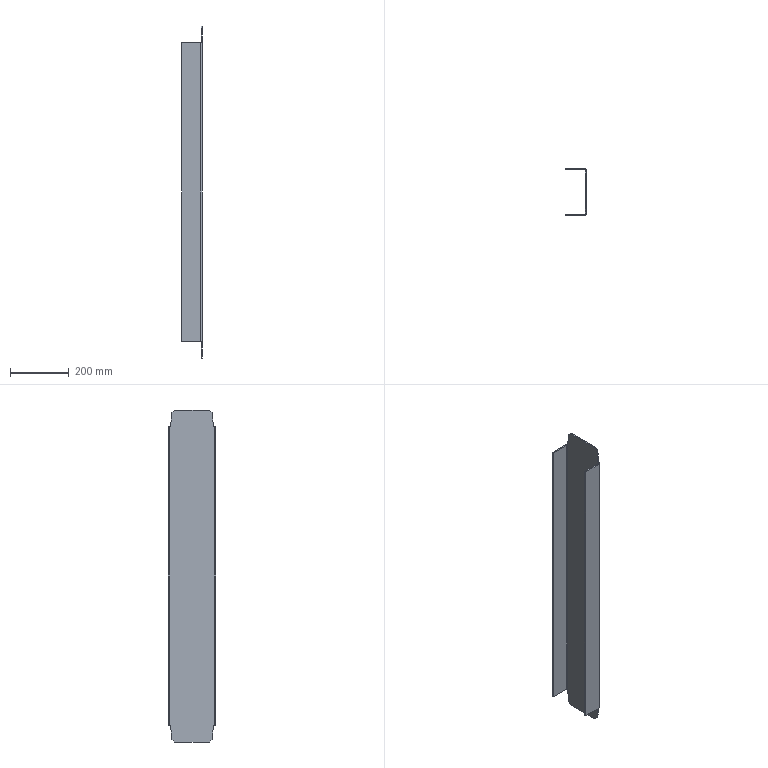Part | SolidWorks | 1 solid | 38 faces | box 70 x 160 x 1127 mm | volume 1236525 mm3 | plane 34 | cylinder 4 | commonest cylinder face diameters 2 x2 10 x2
STEP:
#1=CARTESIAN_POINT('',(-70.,4.,-507.));
#2=VERTEX_POINT('',#1);
#3=CARTESIAN_POINT('',(-5.,4.,-507.));
#4=VERTEX_POINT('',#3);
#5=CARTESIAN_POINT('',(0.,4.,-507.));
#6=DIRECTION('',(1.,0.,0.));
#7=VECTOR('',#6,1000.);
#8=LINE('',#5,#7);
#9=EDGE_CURVE('',#2,#4,#8,.T.);
#10=ORIENTED_EDGE('',*,*,#9,.F.);
#11=CARTESIAN_POINT('',(-70.,4.,507.));
#12=VERTEX_POINT('',#11);
#13=CARTESIAN_POINT('',(-70.,4.,563.5));
#14=DIRECTION('',(0.,0.,-1.));
#15=VECTOR('',#14,1000.);
#16=LINE('',#13,#15);
#17=EDGE_CURVE('',#12,#2,#16,.T.);
#18=ORIENTED_EDGE('',*,*,#17,.F.);
#19=CARTESIAN_POINT('',(-5.,4.,507.));
#20=VERTEX_POINT('',#19);
#21=CARTESIAN_POINT('',(0.,4.,507.));
#22=DIRECTION('',(1.,0.,0.));
#23=VECTOR('',#22,1000.);
#24=LINE('',#21,#23);
#25=EDGE_CURVE('',#12,#20,#24,.T.);
#26=ORIENTED_EDGE('',*,*,#25,.T.);
#27=CARTESIAN_POINT('',(-5.,4.,563.5));
#28=DIRECTION('',(0.,0.,-1.));
#29=VECTOR('',#28,1000.);
#30=LINE('',#27,#29);
#31=EDGE_CURVE('',#20,#4,#30,.T.);
#32=ORIENTED_EDGE('',*,*,#31,.T.);
#33=EDGE_LOOP('',(#10,#18,#26,#32));
#34=FACE_OUTER_BOUND('',#33,.T.);
#35=CARTESIAN_POINT('',(0.,4.,563.5));
#36=DIRECTION('',(0.,-1.,0.));
#37=DIRECTION('',(1.,0.,0.));
#38=AXIS2_PLACEMENT_3D('',#35,#36,#37);
#39=PLANE('',#38);
#40=ADVANCED_FACE('',(#34),#39,.F.);
#41=ORIENTED_EDGE('',*,*,#17,.T.);
#42=CARTESIAN_POINT('',(-70.,0.,-507.));
#43=VERTEX_POINT('',#42);
#44=CARTESIAN_POINT('',(-70.,0.,-507.));
#45=DIRECTION('',(0.,1.,0.));
#46=VECTOR('',#45,1000.);
#47=LINE('',#44,#46);
#48=EDGE_CURVE('',#43,#2,#47,.T.);
#49=ORIENTED_EDGE('',*,*,#48,.F.);
#50=CARTESIAN_POINT('',(-70.,0.,507.));
#51=VERTEX_POINT('',#50);
#52=CARTESIAN_POINT('',(-70.,0.,563.5));
#53=DIRECTION('',(0.,0.,-1.));
#54=VECTOR('',#53,1000.);
#55=LINE('',#52,#54);
#56=EDGE_CURVE('',#51,#43,#55,.T.);
#57=ORIENTED_EDGE('',*,*,#56,.F.);
#58=CARTESIAN_POINT('',(-70.,0.,507.));
#59=DIRECTION('',(0.,1.,0.));
#60=VECTOR('',#59,1000.);
#61=LINE('',#58,#60);
#62=EDGE_CURVE('',#51,#12,#61,.T.);
#63=ORIENTED_EDGE('',*,*,#62,.T.);
#64=EDGE_LOOP('',(#41,#49,#57,#63));
#65=FACE_OUTER_BOUND('',#64,.T.);
#66=CARTESIAN_POINT('',(-70.,0.,563.5));
#67=DIRECTION('',(-1.,0.,0.));
#68=DIRECTION('',(0.,0.,1.));
#69=AXIS2_PLACEMENT_3D('',#66,#67,#68);
#70=PLANE('',#69);
#71=ADVANCED_FACE('',(#65),#70,.T.);
#72=ORIENTED_EDGE('',*,*,#56,.T.);
#73=CARTESIAN_POINT('',(-5.,0.,-507.));
#74=VERTEX_POINT('',#73);
#75=CARTESIAN_POINT('',(0.,0.,-507.));
#76=DIRECTION('',(1.,0.,0.));
#77=VECTOR('',#76,1000.);
#78=LINE('',#75,#77);
#79=EDGE_CURVE('',#43,#74,#78,.T.);
#80=ORIENTED_EDGE('',*,*,#79,.T.);
#81=CARTESIAN_POINT('',(-5.,0.,507.));
#82=VERTEX_POINT('',#81);
#83=CARTESIAN_POINT('',(-5.,0.,563.5));
#84=DIRECTION('',(0.,0.,-1.));
#85=VECTOR('',#84,1000.);
#86=LINE('',#83,#85);
#87=EDGE_CURVE('',#82,#74,#86,.T.);
#88=ORIENTED_EDGE('',*,*,#87,.F.);
#89=CARTESIAN_POINT('',(0.,0.,507.));
#90=DIRECTION('',(1.,0.,0.));
#91=VECTOR('',#90,1000.);
#92=LINE('',#89,#91);
#93=EDGE_CURVE('',#51,#82,#92,.T.);
#94=ORIENTED_EDGE('',*,*,#93,.F.);
#95=EDGE_LOOP('',(#72,#80,#88,#94));
#96=FACE_OUTER_BOUND('',#95,.T.);
#97=CARTESIAN_POINT('',(0.,0.,563.5));
#98=DIRECTION('',(0.,-1.,0.));
#99=DIRECTION('',(1.,0.,0.));
#100=AXIS2_PLACEMENT_3D('',#97,#98,#99);
#101=PLANE('',#100);
#102=ADVANCED_FACE('',(#96),#101,.T.);
#103=ORIENTED_EDGE('',*,*,#87,.T.);
#104=CARTESIAN_POINT('',(0.,5.,-507.));
#105=VERTEX_POINT('',#104);
#106=CARTESIAN_POINT('',(-5.,5.,-507.));
#107=DIRECTION('',(0.,0.,1.));
#108=DIRECTION('',(0.,1.,0.));
#109=AXIS2_PLACEMENT_3D('',#106,#107,#108);
#110=CIRCLE('',#109,5.);
#111=EDGE_CURVE('',#74,#105,#110,.T.);
#112=ORIENTED_EDGE('',*,*,#111,.T.);
#113=CARTESIAN_POINT('',(0.,5.,507.));
#114=VERTEX_POINT('',#113);
#115=CARTESIAN_POINT('',(0.,5.,563.5));
#116=DIRECTION('',(0.,0.,-1.));
#117=VECTOR('',#116,1000.);
#118=LINE('',#115,#117);
#119=EDGE_CURVE('',#114,#105,#118,.T.);
#120=ORIENTED_EDGE('',*,*,#119,.F.);
#121=CARTESIAN_POINT('',(-5.,5.,507.));
#122=DIRECTION('',(0.,0.,1.));
#123=DIRECTION('',(-1.,0.,0.));
#124=AXIS2_PLACEMENT_3D('',#121,#122,#123);
#125=CIRCLE('',#124,5.);
#126=EDGE_CURVE('',#82,#114,#125,.T.);
#127=ORIENTED_EDGE('',*,*,#126,.F.);
#128=EDGE_LOOP('',(#103,#112,#120,#127));
#129=FACE_OUTER_BOUND('',#128,.T.);
#130=CARTESIAN_POINT('',(-5.,5.,563.5));
#131=DIRECTION('',(0.,0.,-1.));
#132=DIRECTION('',(-1.,0.,0.));
#133=AXIS2_PLACEMENT_3D('',#130,#131,#132);
#134=CYLINDRICAL_SURFACE('',#133,5.);
#135=ADVANCED_FACE('',(#129),#134,.T.);
#136=ORIENTED_EDGE('',*,*,#119,.T.);
#137=CARTESIAN_POINT('',(0.,7.501,-507.));
#138=VERTEX_POINT('',#137);
#139=CARTESIAN_POINT('',(0.,160.,-507.));
#140=DIRECTION('',(0.,1.,0.));
#141=VECTOR('',#140,1000.);
#142=LINE('',#139,#141);
#143=EDGE_CURVE('',#105,#138,#142,.T.);
#144=ORIENTED_EDGE('',*,*,#143,.T.);
#145=CARTESIAN_POINT('',(0.,7.501,-511.477));
#146=VERTEX_POINT('',#145);
#147=CARTESIAN_POINT('',(0.,7.501,563.5));
#148=DIRECTION('',(0.,0.,-1.));
#149=VECTOR('',#148,1000.);
#150=LINE('',#147,#149);
#151=EDGE_CURVE('',#138,#146,#150,.T.);
#152=ORIENTED_EDGE('',*,*,#151,.T.);
#153=CARTESIAN_POINT('',(0.,12.028,-554.545));
#154=VERTEX_POINT('',#153);
#155=CARTESIAN_POINT('',(0.,-102.583,535.901));
#156=DIRECTION('',(0.,0.1045,-0.9945));
#157=VECTOR('',#156,1000.);
#158=LINE('',#155,#157);
#159=EDGE_CURVE('',#146,#154,#158,.T.);
#160=ORIENTED_EDGE('',*,*,#159,.T.);
#161=CARTESIAN_POINT('',(0.,21.973,-563.5));
#162=VERTEX_POINT('',#161);
#163=CARTESIAN_POINT('',(0.,-462.213,-127.537));
#164=DIRECTION('',(0.,0.7431,-0.6691));
#165=VECTOR('',#164,1000.);
#166=LINE('',#163,#165);
#167=EDGE_CURVE('',#154,#162,#166,.T.);
#168=ORIENTED_EDGE('',*,*,#167,.T.);
#169=CARTESIAN_POINT('',(0.,138.027,-563.5));
#170=VERTEX_POINT('',#169);
#171=CARTESIAN_POINT('',(0.,160.,-563.5));
#172=DIRECTION('',(0.,-1.,0.));
#173=VECTOR('',#172,1000.);
#174=LINE('',#171,#173);
#175=EDGE_CURVE('',#170,#162,#174,.T.);
#176=ORIENTED_EDGE('',*,*,#175,.F.);
#177=CARTESIAN_POINT('',(0.,147.972,-554.545));
#178=VERTEX_POINT('',#177);
#179=CARTESIAN_POINT('',(0.,710.575,-47.975));
#180=DIRECTION('',(0.,0.7431,0.6691));
#181=VECTOR('',#180,1000.);
#182=LINE('',#179,#181);
#183=EDGE_CURVE('',#170,#178,#182,.T.);
#184=ORIENTED_EDGE('',*,*,#183,.T.);
#185=CARTESIAN_POINT('',(0.,152.499,-511.477));
#186=VERTEX_POINT('',#185);
#187=CARTESIAN_POINT('',(0.,264.331,552.534));
#188=DIRECTION('',(0.,0.1045,0.9945));
#189=VECTOR('',#188,1000.);
#190=LINE('',#187,#189);
#191=EDGE_CURVE('',#178,#186,#190,.T.);
#192=ORIENTED_EDGE('',*,*,#191,.T.);
#193=CARTESIAN_POINT('',(0.,152.499,-507.));
#194=VERTEX_POINT('',#193);
#195=CARTESIAN_POINT('',(0.,152.499,563.5));
#196=DIRECTION('',(0.,0.,1.));
#197=VECTOR('',#196,1000.);
#198=LINE('',#195,#197);
#199=EDGE_CURVE('',#186,#194,#198,.T.);
#200=ORIENTED_EDGE('',*,*,#199,.T.);
#201=CARTESIAN_POINT('',(0.,155.,-507.));
#202=VERTEX_POINT('',#201);
#203=CARTESIAN_POINT('',(0.,160.,-507.));
#204=DIRECTION('',(0.,1.,0.));
#205=VECTOR('',#204,1000.);
#206=LINE('',#203,#205);
#207=EDGE_CURVE('',#194,#202,#206,.T.);
#208=ORIENTED_EDGE('',*,*,#207,.T.);
#209=CARTESIAN_POINT('',(0.,155.,507.));
#210=VERTEX_POINT('',#209);
#211=CARTESIAN_POINT('',(0.,155.,563.5));
#212=DIRECTION('',(0.,0.,-1.));
#213=VECTOR('',#212,1000.);
#214=LINE('',#211,#213);
#215=EDGE_CURVE('',#210,#202,#214,.T.);
#216=ORIENTED_EDGE('',*,*,#215,.F.);
#217=CARTESIAN_POINT('',(0.,152.499,507.));
#218=VERTEX_POINT('',#217);
#219=CARTESIAN_POINT('',(0.,160.,507.));
#220=DIRECTION('',(0.,1.,0.));
#221=VECTOR('',#220,1000.);
#222=LINE('',#219,#221);
#223=EDGE_CURVE('',#218,#210,#222,.T.);
#224=ORIENTED_EDGE('',*,*,#223,.F.);
#225=CARTESIAN_POINT('',(0.,152.499,511.477));
#226=VERTEX_POINT('',#225);
#227=CARTESIAN_POINT('',(0.,152.499,563.5));
#228=DIRECTION('',(0.,0.,-1.));
#229=VECTOR('',#228,1000.);
#230=LINE('',#227,#229);
#231=EDGE_CURVE('',#226,#218,#230,.T.);
#232=ORIENTED_EDGE('',*,*,#231,.F.);
#233=CARTESIAN_POINT('',(0.,147.972,554.545));
#234=VERTEX_POINT('',#233);
#235=CARTESIAN_POINT('',(0.,147.173,562.152));
#236=DIRECTION('',(0.,0.1045,-0.9945));
#237=VECTOR('',#236,1000.);
#238=LINE('',#235,#237);
#239=EDGE_CURVE('',#234,#226,#238,.T.);
#240=ORIENTED_EDGE('',*,*,#239,.F.);
#241=CARTESIAN_POINT('',(0.,138.027,563.5));
#242=VERTEX_POINT('',#241);
#243=CARTESIAN_POINT('',(0.,150.162,552.574));
#244=DIRECTION('',(0.,0.7431,-0.6691));
#245=VECTOR('',#244,1000.);
#246=LINE('',#243,#245);
#247=EDGE_CURVE('',#242,#234,#246,.T.);
#248=ORIENTED_EDGE('',*,*,#247,.F.);
#249=CARTESIAN_POINT('',(0.,21.973,563.5));
#250=VERTEX_POINT('',#249);
#251=CARTESIAN_POINT('',(0.,160.,563.5));
#252=DIRECTION('',(0.,-1.,0.));
#253=VECTOR('',#252,1000.);
#254=LINE('',#251,#253);
#255=EDGE_CURVE('',#242,#250,#254,.T.);
#256=ORIENTED_EDGE('',*,*,#255,.T.);
#257=CARTESIAN_POINT('',(0.,12.028,554.545));
#258=VERTEX_POINT('',#257);
#259=CARTESIAN_POINT('',(0.,98.2,632.135));
#260=DIRECTION('',(0.,0.7431,0.6691));
#261=VECTOR('',#260,1000.);
#262=LINE('',#259,#261);
#263=EDGE_CURVE('',#258,#250,#262,.T.);
#264=ORIENTED_EDGE('',*,*,#263,.F.);
#265=CARTESIAN_POINT('',(0.,7.501,511.477));
#266=VERTEX_POINT('',#265);
#267=CARTESIAN_POINT('',(0.,14.576,578.785));
#268=DIRECTION('',(0.,0.1045,0.9945));
#269=VECTOR('',#268,1000.);
#270=LINE('',#267,#269);
#271=EDGE_CURVE('',#266,#258,#270,.T.);
#272=ORIENTED_EDGE('',*,*,#271,.F.);
#273=CARTESIAN_POINT('',(0.,7.501,507.));
#274=VERTEX_POINT('',#273);
#275=CARTESIAN_POINT('',(0.,7.501,563.5));
#276=DIRECTION('',(0.,0.,1.));
#277=VECTOR('',#276,1000.);
#278=LINE('',#275,#277);
#279=EDGE_CURVE('',#274,#266,#278,.T.);
#280=ORIENTED_EDGE('',*,*,#279,.F.);
#281=CARTESIAN_POINT('',(0.,160.,507.));
#282=DIRECTION('',(0.,1.,0.));
#283=VECTOR('',#282,1000.);
#284=LINE('',#281,#283);
#285=EDGE_CURVE('',#114,#274,#284,.T.);
#286=ORIENTED_EDGE('',*,*,#285,.F.);
#287=EDGE_LOOP('',(#136,#144,#152,#160,#168,#176,#184,#192,#200,#208,#216,#224,#232,#240,#248,#256,#264,#272,#280,#286));
#288=FACE_OUTER_BOUND('',#287,.T.);
#289=CARTESIAN_POINT('',(0.,160.,563.5));
#290=DIRECTION('',(1.,0.,0.));
#291=DIRECTION('',(0.,1.,0.));
#292=AXIS2_PLACEMENT_3D('',#289,#290,#291);
#293=PLANE('',#292);
#294=ADVANCED_FACE('',(#288),#293,.T.);
#295=ORIENTED_EDGE('',*,*,#215,.T.);
#296=CARTESIAN_POINT('',(-5.,160.,-507.));
#297=VERTEX_POINT('',#296);
#298=CARTESIAN_POINT('',(-5.,155.,-507.));
#299=DIRECTION('',(0.,0.,1.));
#300=DIRECTION('',(-1.,0.,0.));
#301=AXIS2_PLACEMENT_3D('',#298,#299,#300);
#302=CIRCLE('',#301,5.);
#303=EDGE_CURVE('',#202,#297,#302,.T.);
#304=ORIENTED_EDGE('',*,*,#303,.T.);
#305=CARTESIAN_POINT('',(-5.,160.,507.));
#306=VERTEX_POINT('',#305);
#307=CARTESIAN_POINT('',(-5.,160.,563.5));
#308=DIRECTION('',(0.,0.,-1.));
#309=VECTOR('',#308,1000.);
#310=LINE('',#307,#309);
#311=EDGE_CURVE('',#306,#297,#310,.T.);
#312=ORIENTED_EDGE('',*,*,#311,.F.);
#313=CARTESIAN_POINT('',(-5.,155.,507.));
#314=DIRECTION('',(0.,0.,1.));
#315=DIRECTION('',(-1.,0.,0.));
#316=AXIS2_PLACEMENT_3D('',#313,#314,#315);
#317=CIRCLE('',#316,5.);
#318=EDGE_CURVE('',#210,#306,#317,.T.);
#319=ORIENTED_EDGE('',*,*,#318,.F.);
#320=EDGE_LOOP('',(#295,#304,#312,#319));
#321=FACE_OUTER_BOUND('',#320,.T.);
#322=CARTESIAN_POINT('',(-5.,155.,563.5));
#323=DIRECTION('',(0.,0.,-1.));
#324=DIRECTION('',(-1.,0.,0.));
#325=AXIS2_PLACEMENT_3D('',#322,#323,#324);
#326=CYLINDRICAL_SURFACE('',#325,5.);
#327=ADVANCED_FACE('',(#321),#326,.T.);
#328=ORIENTED_EDGE('',*,*,#311,.T.);
#329=CARTESIAN_POINT('',(-70.,160.,-507.));
#330=VERTEX_POINT('',#329);
#331=CARTESIAN_POINT('',(-70.,160.,-507.));
#332=DIRECTION('',(-1.,0.,0.));
#333=VECTOR('',#332,1000.);
#334=LINE('',#331,#333);
#335=EDGE_CURVE('',#297,#330,#334,.T.);
#336=ORIENTED_EDGE('',*,*,#335,.T.);
#337=CARTESIAN_POINT('',(-70.,160.,507.));
#338=VERTEX_POINT('',#337);
#339=CARTESIAN_POINT('',(-70.,160.,563.5));
#340=DIRECTION('',(0.,0.,-1.));
#341=VECTOR('',#340,1000.);
#342=LINE('',#339,#341);
#343=EDGE_CURVE('',#338,#330,#342,.T.);
#344=ORIENTED_EDGE('',*,*,#343,.F.);
#345=CARTESIAN_POINT('',(-70.,160.,507.));
#346=DIRECTION('',(-1.,0.,0.));
#347=VECTOR('',#346,1000.);
#348=LINE('',#345,#347);
#349=EDGE_CURVE('',#306,#338,#348,.T.);
#350=ORIENTED_EDGE('',*,*,#349,.F.);
#351=EDGE_LOOP('',(#328,#336,#344,#350));
#352=FACE_OUTER_BOUND('',#351,.T.);
#353=CARTESIAN_POINT('',(-70.,160.,563.5));
#354=DIRECTION('',(0.,1.,0.));
#355=DIRECTION('',(0.,0.,1.));
#356=AXIS2_PLACEMENT_3D('',#353,#354,#355);
#357=PLANE('',#356);
#358=ADVANCED_FACE('',(#352),#357,.T.);
#359=ORIENTED_EDGE('',*,*,#343,.T.);
#360=CARTESIAN_POINT('',(-70.,156.,-507.));
#361=VERTEX_POINT('',#360);
#362=CARTESIAN_POINT('',(-70.,160.,-507.));
#363=DIRECTION('',(0.,-1.,0.));
#364=VECTOR('',#363,1000.);
#365=LINE('',#362,#364);
#366=EDGE_CURVE('',#330,#361,#365,.T.);
#367=ORIENTED_EDGE('',*,*,#366,.T.);
#368=CARTESIAN_POINT('',(-70.,156.,507.));
#369=VERTEX_POINT('',#368);
#370=CARTESIAN_POINT('',(-70.,156.,563.5));
#371=DIRECTION('',(0.,0.,-1.));
#372=VECTOR('',#371,1000.);
#373=LINE('',#370,#372);
#374=EDGE_CURVE('',#369,#361,#373,.T.);
#375=ORIENTED_EDGE('',*,*,#374,.F.);
#376=CARTESIAN_POINT('',(-70.,156.,507.));
#377=DIRECTION('',(0.,1.,0.));
#378=VECTOR('',#377,1000.);
#379=LINE('',#376,#378);
#380=EDGE_CURVE('',#369,#338,#379,.T.);
#381=ORIENTED_EDGE('',*,*,#380,.T.);
#382=EDGE_LOOP('',(#359,#367,#375,#381));
#383=FACE_OUTER_BOUND('',#382,.T.);
#384=CARTESIAN_POINT('',(-70.,156.,563.5));
#385=DIRECTION('',(-1.,0.,0.));
#386=DIRECTION('',(0.,0.,1.));
#387=AXIS2_PLACEMENT_3D('',#384,#385,#386);
#388=PLANE('',#387);
#389=ADVANCED_FACE('',(#383),#388,.T.);
#390=CARTESIAN_POINT('',(-5.,156.,-507.));
#391=VERTEX_POINT('',#390);
#392=CARTESIAN_POINT('',(-70.,156.,-507.));
#393=DIRECTION('',(-1.,0.,0.));
#394=VECTOR('',#393,1000.);
#395=LINE('',#392,#394);
#396=EDGE_CURVE('',#391,#361,#395,.T.);
#397=ORIENTED_EDGE('',*,*,#396,.F.);
#398=CARTESIAN_POINT('',(-5.,156.,507.));
#399=VERTEX_POINT('',#398);
#400=CARTESIAN_POINT('',(-5.,156.,563.5));
#401=DIRECTION('',(0.,0.,-1.));
#402=VECTOR('',#401,1000.);
#403=LINE('',#400,#402);
#404=EDGE_CURVE('',#399,#391,#403,.T.);
#405=ORIENTED_EDGE('',*,*,#404,.F.);
#406=CARTESIAN_POINT('',(-70.,156.,507.));
#407=DIRECTION('',(-1.,0.,0.));
#408=VECTOR('',#407,1000.);
#409=LINE('',#406,#408);
#410=EDGE_CURVE('',#399,#369,#409,.T.);
#411=ORIENTED_EDGE('',*,*,#410,.T.);
#412=ORIENTED_EDGE('',*,*,#374,.T.);
#413=EDGE_LOOP('',(#397,#405,#411,#412));
#414=FACE_OUTER_BOUND('',#413,.T.);
#415=CARTESIAN_POINT('',(-70.,156.,563.5));
#416=DIRECTION('',(0.,1.,0.));
#417=DIRECTION('',(0.,0.,1.));
#418=AXIS2_PLACEMENT_3D('',#415,#416,#417);
#419=PLANE('',#418);
#420=ADVANCED_FACE('',(#414),#419,.F.);
#421=CARTESIAN_POINT('',(-4.,155.,-507.));
#422=VERTEX_POINT('',#421);
#423=CARTESIAN_POINT('',(-5.,155.,-507.));
#424=DIRECTION('',(0.,0.,1.));
#425=DIRECTION('',(-1.,0.,0.));
#426=AXIS2_PLACEMENT_3D('',#423,#424,#425);
#427=CIRCLE('',#426,1.);
#428=EDGE_CURVE('',#422,#391,#427,.T.);
#429=ORIENTED_EDGE('',*,*,#428,.F.);
#430=CARTESIAN_POINT('',(-4.,155.,507.));
#431=VERTEX_POINT('',#430);
#432=CARTESIAN_POINT('',(-4.,155.,563.5));
#433=DIRECTION('',(0.,0.,-1.));
#434=VECTOR('',#433,1000.);
#435=LINE('',#432,#434);
#436=EDGE_CURVE('',#431,#422,#435,.T.);
#437=ORIENTED_EDGE('',*,*,#436,.F.);
#438=CARTESIAN_POINT('',(-5.,155.,507.));
#439=DIRECTION('',(0.,0.,1.));
#440=DIRECTION('',(-1.,0.,0.));
#441=AXIS2_PLACEMENT_3D('',#438,#439,#440);
#442=CIRCLE('',#441,1.);
#443=EDGE_CURVE('',#431,#399,#442,.T.);
#444=ORIENTED_EDGE('',*,*,#443,.T.);
#445=ORIENTED_EDGE('',*,*,#404,.T.);
#446=EDGE_LOOP('',(#429,#437,#444,#445));
#447=FACE_OUTER_BOUND('',#446,.T.);
#448=CARTESIAN_POINT('',(-5.,155.,563.5));
#449=DIRECTION('',(0.,0.,-1.));
#450=DIRECTION('',(-1.,0.,0.));
#451=AXIS2_PLACEMENT_3D('',#448,#449,#450);
#452=CYLINDRICAL_SURFACE('',#451,1.);
#453=ADVANCED_FACE('',(#447),#452,.F.);
#454=CARTESIAN_POINT('',(-4.,5.,-507.));
#455=VERTEX_POINT('',#454);
#456=CARTESIAN_POINT('',(-4.,7.501,-507.));
#457=VERTEX_POINT('',#456);
#458=CARTESIAN_POINT('',(-4.,160.,-507.));
#459=DIRECTION('',(0.,1.,0.));
#460=VECTOR('',#459,1000.);
#461=LINE('',#458,#460);
#462=EDGE_CURVE('',#455,#457,#461,.T.);
#463=ORIENTED_EDGE('',*,*,#462,.F.);
#464=CARTESIAN_POINT('',(-4.,5.,507.));
#465=VERTEX_POINT('',#464);
#466=CARTESIAN_POINT('',(-4.,5.,563.5));
#467=DIRECTION('',(0.,0.,-1.));
#468=VECTOR('',#467,1000.);
#469=LINE('',#466,#468);
#470=EDGE_CURVE('',#465,#455,#469,.T.);
#471=ORIENTED_EDGE('',*,*,#470,.F.);
#472=CARTESIAN_POINT('',(-4.,7.501,507.));
#473=VERTEX_POINT('',#472);
#474=CARTESIAN_POINT('',(-4.,160.,507.));
#475=DIRECTION('',(0.,1.,0.));
#476=VECTOR('',#475,1000.);
#477=LINE('',#474,#476);
#478=EDGE_CURVE('',#465,#473,#477,.T.);
#479=ORIENTED_EDGE('',*,*,#478,.T.);
#480=CARTESIAN_POINT('',(-4.,7.501,511.477));
#481=VERTEX_POINT('',#480);
#482=CARTESIAN_POINT('',(-4.,7.501,563.5));
#483=DIRECTION('',(0.,0.,1.));
#484=VECTOR('',#483,1000.);
#485=LINE('',#482,#484);
#486=EDGE_CURVE('',#473,#481,#485,.T.);
#487=ORIENTED_EDGE('',*,*,#486,.T.);
#488=CARTESIAN_POINT('',(-4.,12.028,554.545));
#489=VERTEX_POINT('',#488);
#490=CARTESIAN_POINT('',(-4.,14.576,578.785));
#491=DIRECTION('',(0.,0.1045,0.9945));
#492=VECTOR('',#491,1000.);
#493=LINE('',#490,#492);
#494=EDGE_CURVE('',#481,#489,#493,.T.);
#495=ORIENTED_EDGE('',*,*,#494,.T.);
#496=CARTESIAN_POINT('',(-4.,21.973,563.5));
#497=VERTEX_POINT('',#496);
#498=CARTESIAN_POINT('',(-4.,98.2,632.135));
#499=DIRECTION('',(0.,0.7431,0.6691));
#500=VECTOR('',#499,1000.);
#501=LINE('',#498,#500);
#502=EDGE_CURVE('',#489,#497,#501,.T.);
#503=ORIENTED_EDGE('',*,*,#502,.T.);
#504=CARTESIAN_POINT('',(-4.,138.027,563.5));
#505=VERTEX_POINT('',#504);
#506=CARTESIAN_POINT('',(-4.,160.,563.5));
#507=DIRECTION('',(0.,-1.,0.));
#508=VECTOR('',#507,1000.);
#509=LINE('',#506,#508);
#510=EDGE_CURVE('',#505,#497,#509,.T.);
#511=ORIENTED_EDGE('',*,*,#510,.F.);
#512=CARTESIAN_POINT('',(-4.,147.972,554.545));
#513=VERTEX_POINT('',#512);
#514=CARTESIAN_POINT('',(-4.,150.162,552.574));
#515=DIRECTION('',(0.,0.7431,-0.6691));
#516=VECTOR('',#515,1000.);
#517=LINE('',#514,#516);
#518=EDGE_CURVE('',#505,#513,#517,.T.);
#519=ORIENTED_EDGE('',*,*,#518,.T.);
#520=CARTESIAN_POINT('',(-4.,152.499,511.477));
#521=VERTEX_POINT('',#520);
#522=CARTESIAN_POINT('',(-4.,147.173,562.152));
#523=DIRECTION('',(0.,0.1045,-0.9945));
#524=VECTOR('',#523,1000.);
#525=LINE('',#522,#524);
#526=EDGE_CURVE('',#513,#521,#525,.T.);
#527=ORIENTED_EDGE('',*,*,#526,.T.);
#528=CARTESIAN_POINT('',(-4.,152.499,507.));
#529=VERTEX_POINT('',#528);
#530=CARTESIAN_POINT('',(-4.,152.499,563.5));
#531=DIRECTION('',(0.,0.,-1.));
#532=VECTOR('',#531,1000.);
#533=LINE('',#530,#532);
#534=EDGE_CURVE('',#521,#529,#533,.T.);
#535=ORIENTED_EDGE('',*,*,#534,.T.);
#536=CARTESIAN_POINT('',(-4.,160.,507.));
#537=DIRECTION('',(0.,1.,0.));
#538=VECTOR('',#537,1000.);
#539=LINE('',#536,#538);
#540=EDGE_CURVE('',#529,#431,#539,.T.);
#541=ORIENTED_EDGE('',*,*,#540,.T.);
#542=ORIENTED_EDGE('',*,*,#436,.T.);
#543=CARTESIAN_POINT('',(-4.,152.499,-507.));
#544=VERTEX_POINT('',#543);
#545=CARTESIAN_POINT('',(-4.,160.,-507.));
#546=DIRECTION('',(0.,1.,0.));
#547=VECTOR('',#546,1000.);
#548=LINE('',#545,#547);
#549=EDGE_CURVE('',#544,#422,#548,.T.);
#550=ORIENTED_EDGE('',*,*,#549,.F.);
#551=CARTESIAN_POINT('',(-4.,152.499,-511.477));
#552=VERTEX_POINT('',#551);
#553=CARTESIAN_POINT('',(-4.,152.499,563.5));
#554=DIRECTION('',(0.,0.,1.));
#555=VECTOR('',#554,1000.);
#556=LINE('',#553,#555);
#557=EDGE_CURVE('',#552,#544,#556,.T.);
#558=ORIENTED_EDGE('',*,*,#557,.F.);
#559=CARTESIAN_POINT('',(-4.,147.972,-554.545));
#560=VERTEX_POINT('',#559);
#561=CARTESIAN_POINT('',(-4.,264.331,552.534));
#562=DIRECTION('',(0.,0.1045,0.9945));
#563=VECTOR('',#562,1000.);
#564=LINE('',#561,#563);
#565=EDGE_CURVE('',#560,#552,#564,.T.);
#566=ORIENTED_EDGE('',*,*,#565,.F.);
#567=CARTESIAN_POINT('',(-4.,138.027,-563.5));
#568=VERTEX_POINT('',#567);
#569=CARTESIAN_POINT('',(-4.,710.575,-47.975));
#570=DIRECTION('',(0.,0.7431,0.6691));
#571=VECTOR('',#570,1000.);
#572=LINE('',#569,#571);
#573=EDGE_CURVE('',#568,#560,#572,.T.);
#574=ORIENTED_EDGE('',*,*,#573,.F.);
#575=CARTESIAN_POINT('',(-4.,21.973,-563.5));
#576=VERTEX_POINT('',#575);
#577=CARTESIAN_POINT('',(-4.,160.,-563.5));
#578=DIRECTION('',(0.,-1.,0.));
#579=VECTOR('',#578,1000.);
#580=LINE('',#577,#579);
#581=EDGE_CURVE('',#568,#576,#580,.T.);
#582=ORIENTED_EDGE('',*,*,#581,.T.);
#583=CARTESIAN_POINT('',(-4.,12.028,-554.545));
#584=VERTEX_POINT('',#583);
#585=CARTESIAN_POINT('',(-4.,-462.213,-127.537));
#586=DIRECTION('',(0.,0.7431,-0.6691));
#587=VECTOR('',#586,1000.);
#588=LINE('',#585,#587);
#589=EDGE_CURVE('',#584,#576,#588,.T.);
#590=ORIENTED_EDGE('',*,*,#589,.F.);
#591=CARTESIAN_POINT('',(-4.,7.501,-511.477));
#592=VERTEX_POINT('',#591);
#593=CARTESIAN_POINT('',(-4.,-102.583,535.901));
#594=DIRECTION('',(0.,0.1045,-0.9945));
#595=VECTOR('',#594,1000.);
#596=LINE('',#593,#595);
#597=EDGE_CURVE('',#592,#584,#596,.T.);
#598=ORIENTED_EDGE('',*,*,#597,.F.);
#599=CARTESIAN_POINT('',(-4.,7.501,563.5));
#600=DIRECTION('',(0.,0.,-1.));
#601=VECTOR('',#600,1000.);
#602=LINE('',#599,#601);
#603=EDGE_CURVE('',#457,#592,#602,.T.);
#604=ORIENTED_EDGE('',*,*,#603,.F.);
#605=EDGE_LOOP('',(#463,#471,#479,#487,#495,#503,#511,#519,#527,#535,#541,#542,#550,#558,#566,#574,#582,#590,#598,#604));
#606=FACE_OUTER_BOUND('',#605,.T.);
#607=CARTESIAN_POINT('',(-4.,160.,563.5));
#608=DIRECTION('',(1.,0.,0.));
#609=DIRECTION('',(0.,1.,0.));
#610=AXIS2_PLACEMENT_3D('',#607,#608,#609);
#611=PLANE('',#610);
#612=ADVANCED_FACE('',(#606),#611,.F.);
#613=CARTESIAN_POINT('',(-5.,5.,-507.));
#614=DIRECTION('',(0.,0.,1.));
#615=DIRECTION('',(-1.,0.,0.));
#616=AXIS2_PLACEMENT_3D('',#613,#614,#615);
#617=CIRCLE('',#616,1.);
#618=EDGE_CURVE('',#4,#455,#617,.T.);
#619=ORIENTED_EDGE('',*,*,#618,.F.);
#620=ORIENTED_EDGE('',*,*,#31,.F.);
#621=CARTESIAN_POINT('',(-5.,5.,507.));
#622=DIRECTION('',(0.,0.,1.));
#623=DIRECTION('',(-1.,0.,0.));
#624=AXIS2_PLACEMENT_3D('',#621,#622,#623);
#625=CIRCLE('',#624,1.);
#626=EDGE_CURVE('',#20,#465,#625,.T.);
#627=ORIENTED_EDGE('',*,*,#626,.T.);
#628=ORIENTED_EDGE('',*,*,#470,.T.);
#629=EDGE_LOOP('',(#619,#620,#627,#628));
#630=FACE_OUTER_BOUND('',#629,.T.);
#631=CARTESIAN_POINT('',(-5.,5.,563.5));
#632=DIRECTION('',(0.,0.,-1.));
#633=DIRECTION('',(-1.,0.,0.));
#634=AXIS2_PLACEMENT_3D('',#631,#632,#633);
#635=CYLINDRICAL_SURFACE('',#634,1.);
#636=ADVANCED_FACE('',(#630),#635,.F.);
#637=ORIENTED_EDGE('',*,*,#175,.T.);
#638=CARTESIAN_POINT('',(-4.,21.973,-563.5));
#639=DIRECTION('',(1.,0.,0.));
#640=VECTOR('',#639,1000.);
#641=LINE('',#638,#640);
#642=EDGE_CURVE('',#576,#162,#641,.T.);
#643=ORIENTED_EDGE('',*,*,#642,.F.);
#644=ORIENTED_EDGE('',*,*,#581,.F.);
#645=CARTESIAN_POINT('',(-4.,138.027,-563.5));
#646=DIRECTION('',(1.,0.,0.));
#647=VECTOR('',#646,1000.);
#648=LINE('',#645,#647);
#649=EDGE_CURVE('',#568,#170,#648,.T.);
#650=ORIENTED_EDGE('',*,*,#649,.T.);
#651=EDGE_LOOP('',(#637,#643,#644,#650));
#652=FACE_OUTER_BOUND('',#651,.T.);
#653=CARTESIAN_POINT('',(-5.,4.,-563.5));
#654=DIRECTION('',(0.,0.,-1.));
#655=DIRECTION('',(-1.,0.,0.));
#656=AXIS2_PLACEMENT_3D('',#653,#654,#655);
#657=PLANE('',#656);
#658=ADVANCED_FACE('',(#652),#657,.T.);
#659=ORIENTED_EDGE('',*,*,#255,.F.);
#660=CARTESIAN_POINT('',(-4.,138.027,563.5));
#661=DIRECTION('',(1.,0.,0.));
#662=VECTOR('',#661,1000.);
#663=LINE('',#660,#662);
#664=EDGE_CURVE('',#505,#242,#663,.T.);
#665=ORIENTED_EDGE('',*,*,#664,.F.);
#666=ORIENTED_EDGE('',*,*,#510,.T.);
#667=CARTESIAN_POINT('',(-4.,21.973,563.5));
#668=DIRECTION('',(1.,0.,0.));
#669=VECTOR('',#668,1000.);
#670=LINE('',#667,#669);
#671=EDGE_CURVE('',#497,#250,#670,.T.);
#672=ORIENTED_EDGE('',*,*,#671,.T.);
#673=EDGE_LOOP('',(#659,#665,#666,#672));
#674=FACE_OUTER_BOUND('',#673,.T.);
#675=CARTESIAN_POINT('',(-5.,156.,563.5));
#676=DIRECTION('',(0.,0.,1.));
#677=DIRECTION('',(1.,0.,0.));
#678=AXIS2_PLACEMENT_3D('',#675,#676,#677);
#679=PLANE('',#678);
#680=ADVANCED_FACE('',(#674),#679,.T.);
#681=ORIENTED_EDGE('',*,*,#93,.T.);
#682=CARTESIAN_POINT('',(-5.,0.,507.));
#683=DIRECTION('',(0.,1.,0.));
#684=VECTOR('',#683,1000.);
#685=LINE('',#682,#684);
#686=EDGE_CURVE('',#82,#20,#685,.T.);
#687=ORIENTED_EDGE('',*,*,#686,.T.);
#688=ORIENTED_EDGE('',*,*,#25,.F.);
#689=ORIENTED_EDGE('',*,*,#62,.F.);
#690=EDGE_LOOP('',(#681,#687,#688,#689));
#691=FACE_OUTER_BOUND('',#690,.T.);
#692=CARTESIAN_POINT('',(0.,0.,507.));
#693=DIRECTION('',(0.,0.,-1.));
#694=DIRECTION('',(1.,0.,0.));
#695=AXIS2_PLACEMENT_3D('',#692,#693,#694);
#696=PLANE('',#695);
#697=ADVANCED_FACE('',(#691),#696,.F.);
#698=CARTESIAN_POINT('',(-4.,7.501,511.477));
#699=DIRECTION('',(1.,0.,0.));
#700=VECTOR('',#699,1000.);
#701=LINE('',#698,#700);
#702=EDGE_CURVE('',#481,#266,#701,.T.);
#703=ORIENTED_EDGE('',*,*,#702,.F.);
#704=ORIENTED_EDGE('',*,*,#486,.F.);
#705=CARTESIAN_POINT('',(-4.,7.501,507.));
#706=DIRECTION('',(1.,0.,0.));
#707=VECTOR('',#706,1000.);
#708=LINE('',#705,#707);
#709=EDGE_CURVE('',#473,#274,#708,.T.);
#710=ORIENTED_EDGE('',*,*,#709,.T.);
#711=ORIENTED_EDGE('',*,*,#279,.T.);
#712=EDGE_LOOP('',(#703,#704,#710,#711));
#713=FACE_OUTER_BOUND('',#712,.T.);
#714=CARTESIAN_POINT('',(-4.,7.501,563.5));
#715=DIRECTION('',(0.,1.,0.));
#716=DIRECTION('',(0.,0.,1.));
#717=AXIS2_PLACEMENT_3D('',#714,#715,#716);
#718=PLANE('',#717);
#719=ADVANCED_FACE('',(#713),#718,.F.);
#720=ORIENTED_EDGE('',*,*,#709,.F.);
#721=ORIENTED_EDGE('',*,*,#478,.F.);
#722=CARTESIAN_POINT('',(-4.,5.,507.));
#723=DIRECTION('',(1.,0.,0.));
#724=VECTOR('',#723,1000.);
#725=LINE('',#722,#724);
#726=EDGE_CURVE('',#465,#114,#725,.T.);
#727=ORIENTED_EDGE('',*,*,#726,.T.);
#728=ORIENTED_EDGE('',*,*,#285,.T.);
#729=EDGE_LOOP('',(#720,#721,#727,#728));
#730=FACE_OUTER_BOUND('',#729,.T.);
#731=CARTESIAN_POINT('',(-4.,160.,507.));
#732=DIRECTION('',(0.,0.,-1.));
#733=DIRECTION('',(0.,1.,0.));
#734=AXIS2_PLACEMENT_3D('',#731,#732,#733);
#735=PLANE('',#734);
#736=ADVANCED_FACE('',(#730),#735,.F.);
#737=ORIENTED_EDGE('',*,*,#671,.F.);
#738=ORIENTED_EDGE('',*,*,#502,.F.);
#739=CARTESIAN_POINT('',(-4.,12.028,554.545));
#740=DIRECTION('',(1.,0.,0.));
#741=VECTOR('',#740,1000.);
#742=LINE('',#739,#741);
#743=EDGE_CURVE('',#489,#258,#742,.T.);
#744=ORIENTED_EDGE('',*,*,#743,.T.);
#745=ORIENTED_EDGE('',*,*,#263,.T.);
#746=EDGE_LOOP('',(#737,#738,#744,#745));
#747=FACE_OUTER_BOUND('',#746,.T.);
#748=CARTESIAN_POINT('',(-4.,98.2,632.135));
#749=DIRECTION('',(0.,0.6691,-0.7431));
#750=DIRECTION('',(0.,0.7431,0.6691));
#751=AXIS2_PLACEMENT_3D('',#748,#749,#750);
#752=PLANE('',#751);
#753=ADVANCED_FACE('',(#747),#752,.F.);
#754=ORIENTED_EDGE('',*,*,#494,.F.);
#755=ORIENTED_EDGE('',*,*,#702,.T.);
#756=ORIENTED_EDGE('',*,*,#271,.T.);
#757=ORIENTED_EDGE('',*,*,#743,.F.);
#758=EDGE_LOOP('',(#754,#755,#756,#757));
#759=FACE_OUTER_BOUND('',#758,.T.);
#760=CARTESIAN_POINT('',(-4.,14.576,578.785));
#761=DIRECTION('',(0.,0.9945,-0.1045));
#762=DIRECTION('',(0.,0.1045,0.9945));
#763=AXIS2_PLACEMENT_3D('',#760,#761,#762);
#764=PLANE('',#763);
#765=ADVANCED_FACE('',(#759),#764,.F.);
#766=ORIENTED_EDGE('',*,*,#726,.F.);
#767=ORIENTED_EDGE('',*,*,#626,.F.);
#768=ORIENTED_EDGE('',*,*,#686,.F.);
#769=ORIENTED_EDGE('',*,*,#126,.T.);
#770=EDGE_LOOP('',(#766,#767,#768,#769));
#771=FACE_OUTER_BOUND('',#770,.T.);
#772=CARTESIAN_POINT('',(-5.,5.,507.));
#773=DIRECTION('',(0.,0.,1.));
#774=DIRECTION('',(1.,0.,0.));
#775=AXIS2_PLACEMENT_3D('',#772,#773,#774);
#776=PLANE('',#775);
#777=ADVANCED_FACE('',(#771),#776,.T.);
#778=CARTESIAN_POINT('',(-4.,155.,507.));
#779=DIRECTION('',(1.,0.,0.));
#780=VECTOR('',#779,1000.);
#781=LINE('',#778,#780);
#782=EDGE_CURVE('',#431,#210,#781,.T.);
#783=ORIENTED_EDGE('',*,*,#782,.F.);
#784=ORIENTED_EDGE('',*,*,#540,.F.);
#785=CARTESIAN_POINT('',(-4.,152.499,507.));
#786=DIRECTION('',(1.,0.,0.));
#787=VECTOR('',#786,1000.);
#788=LINE('',#785,#787);
#789=EDGE_CURVE('',#529,#218,#788,.T.);
#790=ORIENTED_EDGE('',*,*,#789,.T.);
#791=ORIENTED_EDGE('',*,*,#223,.T.);
#792=EDGE_LOOP('',(#783,#784,#790,#791));
#793=FACE_OUTER_BOUND('',#792,.T.);
#794=CARTESIAN_POINT('',(-4.,160.,507.));
#795=DIRECTION('',(0.,0.,-1.));
#796=DIRECTION('',(0.,1.,0.));
#797=AXIS2_PLACEMENT_3D('',#794,#795,#796);
#798=PLANE('',#797);
#799=ADVANCED_FACE('',(#793),#798,.F.);
#800=ORIENTED_EDGE('',*,*,#789,.F.);
#801=ORIENTED_EDGE('',*,*,#534,.F.);
#802=CARTESIAN_POINT('',(-4.,152.499,511.477));
#803=DIRECTION('',(1.,0.,0.));
#804=VECTOR('',#803,1000.);
#805=LINE('',#802,#804);
#806=EDGE_CURVE('',#521,#226,#805,.T.);
#807=ORIENTED_EDGE('',*,*,#806,.T.);
#808=ORIENTED_EDGE('',*,*,#231,.T.);
#809=EDGE_LOOP('',(#800,#801,#807,#808));
#810=FACE_OUTER_BOUND('',#809,.T.);
#811=CARTESIAN_POINT('',(-4.,152.499,563.5));
#812=DIRECTION('',(0.,-1.,0.));
#813=DIRECTION('',(0.,0.,-1.));
#814=AXIS2_PLACEMENT_3D('',#811,#812,#813);
#815=PLANE('',#814);
#816=ADVANCED_FACE('',(#810),#815,.F.);
#817=ORIENTED_EDGE('',*,*,#806,.F.);
#818=ORIENTED_EDGE('',*,*,#526,.F.);
#819=CARTESIAN_POINT('',(-4.,147.972,554.545));
#820=DIRECTION('',(1.,0.,0.));
#821=VECTOR('',#820,1000.);
#822=LINE('',#819,#821);
#823=EDGE_CURVE('',#513,#234,#822,.T.);
#824=ORIENTED_EDGE('',*,*,#823,.T.);
#825=ORIENTED_EDGE('',*,*,#239,.T.);
#826=EDGE_LOOP('',(#817,#818,#824,#825));
#827=FACE_OUTER_BOUND('',#826,.T.);
#828=CARTESIAN_POINT('',(-4.,147.173,562.152));
#829=DIRECTION('',(0.,-0.9945,-0.1045));
#830=DIRECTION('',(0.,0.1045,-0.9945));
#831=AXIS2_PLACEMENT_3D('',#828,#829,#830);
#832=PLANE('',#831);
#833=ADVANCED_FACE('',(#827),#832,.F.);
#834=ORIENTED_EDGE('',*,*,#823,.F.);
#835=ORIENTED_EDGE('',*,*,#518,.F.);
#836=ORIENTED_EDGE('',*,*,#664,.T.);
#837=ORIENTED_EDGE('',*,*,#247,.T.);
#838=EDGE_LOOP('',(#834,#835,#836,#837));
#839=FACE_OUTER_BOUND('',#838,.T.);
#840=CARTESIAN_POINT('',(-4.,150.162,552.574));
#841=DIRECTION('',(0.,-0.6691,-0.7431));
#842=DIRECTION('',(0.,0.7431,-0.6691));
#843=AXIS2_PLACEMENT_3D('',#840,#841,#842);
#844=PLANE('',#843);
#845=ADVANCED_FACE('',(#839),#844,.F.);
#846=ORIENTED_EDGE('',*,*,#318,.T.);
#847=CARTESIAN_POINT('',(-5.,156.,507.));
#848=DIRECTION('',(0.,1.,0.));
#849=VECTOR('',#848,1000.);
#850=LINE('',#847,#849);
#851=EDGE_CURVE('',#399,#306,#850,.T.);
#852=ORIENTED_EDGE('',*,*,#851,.F.);
#853=ORIENTED_EDGE('',*,*,#443,.F.);
#854=ORIENTED_EDGE('',*,*,#782,.T.);
#855=EDGE_LOOP('',(#846,#852,#853,#854));
#856=FACE_OUTER_BOUND('',#855,.T.);
#857=CARTESIAN_POINT('',(-5.,155.,507.));
#858=DIRECTION('',(0.,0.,1.));
#859=DIRECTION('',(1.,0.,0.));
#860=AXIS2_PLACEMENT_3D('',#857,#858,#859);
#861=PLANE('',#860);
#862=ADVANCED_FACE('',(#856),#861,.T.);
#863=ORIENTED_EDGE('',*,*,#380,.F.);
#864=ORIENTED_EDGE('',*,*,#410,.F.);
#865=ORIENTED_EDGE('',*,*,#851,.T.);
#866=ORIENTED_EDGE('',*,*,#349,.T.);
#867=EDGE_LOOP('',(#863,#864,#865,#866));
#868=FACE_OUTER_BOUND('',#867,.T.);
#869=CARTESIAN_POINT('',(-70.,156.,507.));
#870=DIRECTION('',(0.,0.,-1.));
#871=DIRECTION('',(-1.,0.,0.));
#872=AXIS2_PLACEMENT_3D('',#869,#870,#871);
#873=PLANE('',#872);
#874=ADVANCED_FACE('',(#868),#873,.F.);
#875=ORIENTED_EDGE('',*,*,#649,.F.);
#876=ORIENTED_EDGE('',*,*,#573,.T.);
#877=CARTESIAN_POINT('',(-4.,147.972,-554.545));
#878=DIRECTION('',(1.,0.,0.));
#879=VECTOR('',#878,1000.);
#880=LINE('',#877,#879);
#881=EDGE_CURVE('',#560,#178,#880,.T.);
#882=ORIENTED_EDGE('',*,*,#881,.T.);
#883=ORIENTED_EDGE('',*,*,#183,.F.);
#884=EDGE_LOOP('',(#875,#876,#882,#883));
#885=FACE_OUTER_BOUND('',#884,.T.);
#886=CARTESIAN_POINT('',(-4.,710.575,-47.975));
#887=DIRECTION('',(0.,0.6691,-0.7431));
#888=DIRECTION('',(0.,0.7431,0.6691));
#889=AXIS2_PLACEMENT_3D('',#886,#887,#888);
#890=PLANE('',#889);
#891=ADVANCED_FACE('',(#885),#890,.T.);
#892=ORIENTED_EDGE('',*,*,#881,.F.);
#893=ORIENTED_EDGE('',*,*,#565,.T.);
#894=CARTESIAN_POINT('',(-4.,152.499,-511.477));
#895=DIRECTION('',(1.,0.,0.));
#896=VECTOR('',#895,1000.);
#897=LINE('',#894,#896);
#898=EDGE_CURVE('',#552,#186,#897,.T.);
#899=ORIENTED_EDGE('',*,*,#898,.T.);
#900=ORIENTED_EDGE('',*,*,#191,.F.);
#901=EDGE_LOOP('',(#892,#893,#899,#900));
#902=FACE_OUTER_BOUND('',#901,.T.);
#903=CARTESIAN_POINT('',(-4.,264.331,552.534));
#904=DIRECTION('',(0.,0.9945,-0.1045));
#905=DIRECTION('',(0.,0.1045,0.9945));
#906=AXIS2_PLACEMENT_3D('',#903,#904,#905);
#907=PLANE('',#906);
#908=ADVANCED_FACE('',(#902),#907,.T.);
#909=ORIENTED_EDGE('',*,*,#898,.F.);
#910=ORIENTED_EDGE('',*,*,#557,.T.);
#911=CARTESIAN_POINT('',(-4.,152.499,-507.));
#912=DIRECTION('',(1.,0.,0.));
#913=VECTOR('',#912,1000.);
#914=LINE('',#911,#913);
#915=EDGE_CURVE('',#544,#194,#914,.T.);
#916=ORIENTED_EDGE('',*,*,#915,.T.);
#917=ORIENTED_EDGE('',*,*,#199,.F.);
#918=EDGE_LOOP('',(#909,#910,#916,#917));
#919=FACE_OUTER_BOUND('',#918,.T.);
#920=CARTESIAN_POINT('',(-4.,152.499,563.5));
#921=DIRECTION('',(0.,1.,0.));
#922=DIRECTION('',(0.,0.,1.));
#923=AXIS2_PLACEMENT_3D('',#920,#921,#922);
#924=PLANE('',#923);
#925=ADVANCED_FACE('',(#919),#924,.T.);
#926=ORIENTED_EDGE('',*,*,#549,.T.);
#927=CARTESIAN_POINT('',(-4.,155.,-507.));
#928=DIRECTION('',(1.,0.,0.));
#929=VECTOR('',#928,1000.);
#930=LINE('',#927,#929);
#931=EDGE_CURVE('',#422,#202,#930,.T.);
#932=ORIENTED_EDGE('',*,*,#931,.T.);
#933=ORIENTED_EDGE('',*,*,#207,.F.);
#934=ORIENTED_EDGE('',*,*,#915,.F.);
#935=EDGE_LOOP('',(#926,#932,#933,#934));
#936=FACE_OUTER_BOUND('',#935,.T.);
#937=CARTESIAN_POINT('',(-4.,160.,-507.));
#938=DIRECTION('',(0.,0.,-1.));
#939=DIRECTION('',(0.,1.,0.));
#940=AXIS2_PLACEMENT_3D('',#937,#938,#939);
#941=PLANE('',#940);
#942=ADVANCED_FACE('',(#936),#941,.T.);
#943=ORIENTED_EDGE('',*,*,#366,.F.);
#944=ORIENTED_EDGE('',*,*,#335,.F.);
#945=CARTESIAN_POINT('',(-5.,160.,-507.));
#946=DIRECTION('',(0.,-1.,0.));
#947=VECTOR('',#946,1000.);
#948=LINE('',#945,#947);
#949=EDGE_CURVE('',#297,#391,#948,.T.);
#950=ORIENTED_EDGE('',*,*,#949,.T.);
#951=ORIENTED_EDGE('',*,*,#396,.T.);
#952=EDGE_LOOP('',(#943,#944,#950,#951));
#953=FACE_OUTER_BOUND('',#952,.T.);
#954=CARTESIAN_POINT('',(-70.,160.,-507.));
#955=DIRECTION('',(0.,0.,-1.));
#956=DIRECTION('',(-1.,0.,0.));
#957=AXIS2_PLACEMENT_3D('',#954,#955,#956);
#958=PLANE('',#957);
#959=ADVANCED_FACE('',(#953),#958,.T.);
#960=ORIENTED_EDGE('',*,*,#949,.F.);
#961=ORIENTED_EDGE('',*,*,#303,.F.);
#962=ORIENTED_EDGE('',*,*,#931,.F.);
#963=ORIENTED_EDGE('',*,*,#428,.T.);
#964=EDGE_LOOP('',(#960,#961,#962,#963));
#965=FACE_OUTER_BOUND('',#964,.T.);
#966=CARTESIAN_POINT('',(-5.,155.,-507.));
#967=DIRECTION('',(0.,0.,1.));
#968=DIRECTION('',(1.,0.,0.));
#969=AXIS2_PLACEMENT_3D('',#966,#967,#968);
#970=PLANE('',#969);
#971=ADVANCED_FACE('',(#965),#970,.F.);
#972=CARTESIAN_POINT('',(-4.,5.,-507.));
#973=DIRECTION('',(1.,0.,0.));
#974=VECTOR('',#973,1000.);
#975=LINE('',#972,#974);
#976=EDGE_CURVE('',#455,#105,#975,.T.);
#977=ORIENTED_EDGE('',*,*,#976,.F.);
#978=ORIENTED_EDGE('',*,*,#462,.T.);
#979=CARTESIAN_POINT('',(-4.,7.501,-507.));
#980=DIRECTION('',(1.,0.,0.));
#981=VECTOR('',#980,1000.);
#982=LINE('',#979,#981);
#983=EDGE_CURVE('',#457,#138,#982,.T.);
#984=ORIENTED_EDGE('',*,*,#983,.T.);
#985=ORIENTED_EDGE('',*,*,#143,.F.);
#986=EDGE_LOOP('',(#977,#978,#984,#985));
#987=FACE_OUTER_BOUND('',#986,.T.);
#988=CARTESIAN_POINT('',(-4.,160.,-507.));
#989=DIRECTION('',(0.,0.,-1.));
#990=DIRECTION('',(0.,1.,0.));
#991=AXIS2_PLACEMENT_3D('',#988,#989,#990);
#992=PLANE('',#991);
#993=ADVANCED_FACE('',(#987),#992,.T.);
#994=ORIENTED_EDGE('',*,*,#983,.F.);
#995=ORIENTED_EDGE('',*,*,#603,.T.);
#996=CARTESIAN_POINT('',(-4.,7.501,-511.477));
#997=DIRECTION('',(1.,0.,0.));
#998=VECTOR('',#997,1000.);
#999=LINE('',#996,#998);
#1000=EDGE_CURVE('',#592,#146,#999,.T.);
#1001=ORIENTED_EDGE('',*,*,#1000,.T.);
#1002=ORIENTED_EDGE('',*,*,#151,.F.);
#1003=EDGE_LOOP('',(#994,#995,#1001,#1002));
#1004=FACE_OUTER_BOUND('',#1003,.T.);
#1005=CARTESIAN_POINT('',(-4.,7.501,563.5));
#1006=DIRECTION('',(0.,-1.,0.));
#1007=DIRECTION('',(0.,0.,-1.));
#1008=AXIS2_PLACEMENT_3D('',#1005,#1006,#1007);
#1009=PLANE('',#1008);
#1010=ADVANCED_FACE('',(#1004),#1009,.T.);
#1011=ORIENTED_EDGE('',*,*,#1000,.F.);
#1012=ORIENTED_EDGE('',*,*,#597,.T.);
#1013=CARTESIAN_POINT('',(-4.,12.028,-554.545));
#1014=DIRECTION('',(1.,0.,0.));
#1015=VECTOR('',#1014,1000.);
#1016=LINE('',#1013,#1015);
#1017=EDGE_CURVE('',#584,#154,#1016,.T.);
#1018=ORIENTED_EDGE('',*,*,#1017,.T.);
#1019=ORIENTED_EDGE('',*,*,#159,.F.);
#1020=EDGE_LOOP('',(#1011,#1012,#1018,#1019));
#1021=FACE_OUTER_BOUND('',#1020,.T.);
#1022=CARTESIAN_POINT('',(-4.,-102.583,535.901));
#1023=DIRECTION('',(0.,-0.9945,-0.1045));
#1024=DIRECTION('',(0.,0.1045,-0.9945));
#1025=AXIS2_PLACEMENT_3D('',#1022,#1023,#1024);
#1026=PLANE('',#1025);
#1027=ADVANCED_FACE('',(#1021),#1026,.T.);
#1028=ORIENTED_EDGE('',*,*,#589,.T.);
#1029=ORIENTED_EDGE('',*,*,#642,.T.);
#1030=ORIENTED_EDGE('',*,*,#167,.F.);
#1031=ORIENTED_EDGE('',*,*,#1017,.F.);
#1032=EDGE_LOOP('',(#1028,#1029,#1030,#1031));
#1033=FACE_OUTER_BOUND('',#1032,.T.);
#1034=CARTESIAN_POINT('',(-4.,-462.213,-127.537));
#1035=DIRECTION('',(0.,-0.6691,-0.7431));
#1036=DIRECTION('',(0.,0.7431,-0.6691));
#1037=AXIS2_PLACEMENT_3D('',#1034,#1035,#1036);
#1038=PLANE('',#1037);
#1039=ADVANCED_FACE('',(#1033),#1038,.T.);
#1040=ORIENTED_EDGE('',*,*,#976,.T.);
#1041=ORIENTED_EDGE('',*,*,#111,.F.);
#1042=CARTESIAN_POINT('',(-5.,0.,-507.));
#1043=DIRECTION('',(0.,1.,0.));
#1044=VECTOR('',#1043,1000.);
#1045=LINE('',#1042,#1044);
#1046=EDGE_CURVE('',#74,#4,#1045,.T.);
#1047=ORIENTED_EDGE('',*,*,#1046,.T.);
#1048=ORIENTED_EDGE('',*,*,#618,.T.);
#1049=EDGE_LOOP('',(#1040,#1041,#1047,#1048));
#1050=FACE_OUTER_BOUND('',#1049,.T.);
#1051=CARTESIAN_POINT('',(-5.,5.,-507.));
#1052=DIRECTION('',(0.,0.,1.));
#1053=DIRECTION('',(0.,-1.,0.));
#1054=AXIS2_PLACEMENT_3D('',#1051,#1052,#1053);
#1055=PLANE('',#1054);
#1056=ADVANCED_FACE('',(#1050),#1055,.F.);
#1057=ORIENTED_EDGE('',*,*,#1046,.F.);
#1058=ORIENTED_EDGE('',*,*,#79,.F.);
#1059=ORIENTED_EDGE('',*,*,#48,.T.);
#1060=ORIENTED_EDGE('',*,*,#9,.T.);
#1061=EDGE_LOOP('',(#1057,#1058,#1059,#1060));
#1062=FACE_OUTER_BOUND('',#1061,.T.);
#1063=CARTESIAN_POINT('',(0.,0.,-507.));
#1064=DIRECTION('',(0.,0.,-1.));
#1065=DIRECTION('',(1.,0.,0.));
#1066=AXIS2_PLACEMENT_3D('',#1063,#1064,#1065);
#1067=PLANE('',#1066);
#1068=ADVANCED_FACE('',(#1062),#1067,.T.);
#1069=CLOSED_SHELL('',(#40,#71,#102,#135,#294,#327,#358,#389,#420,#453,#612,#636,#658,#680,#697,#719,#736,#753,#765,#777,#799,#816,#833,#845,#862,#874,#891,#908,#925,#942,#959,#971,#993,#1010,#1027,#1039,#1056,#1068));
#1070=MANIFOLD_SOLID_BREP('',#1069);
#1071=CARTESIAN_POINT('',(0.,0.,0.));
#1072=DIRECTION('',(0.,0.,1.));
#1073=DIRECTION('',(1.,0.,0.));
#1074=AXIS2_PLACEMENT_3D('',#1071,#1072,#1073);
#1075=(LENGTH_UNIT()NAMED_UNIT(*)SI_UNIT(.MILLI.,.METRE.));
#1076=UNCERTAINTY_MEASURE_WITH_UNIT(LENGTH_MEASURE(0.00001),#1075,'','');
#1077=(NAMED_UNIT(*)PLANE_ANGLE_UNIT()SI_UNIT($,.RADIAN.));
#1078=(NAMED_UNIT(*)SI_UNIT($,.STERADIAN.)SOLID_ANGLE_UNIT());
#1079=(GEOMETRIC_REPRESENTATION_CONTEXT(3)GLOBAL_UNCERTAINTY_ASSIGNED_CONTEXT((#1076))GLOBAL_UNIT_ASSIGNED_CONTEXT((#1075,#1077,#1078))REPRESENTATION_CONTEXT('',''));
#1080=ADVANCED_BREP_SHAPE_REPRESENTATION('',(#1070,#1074),#1079);